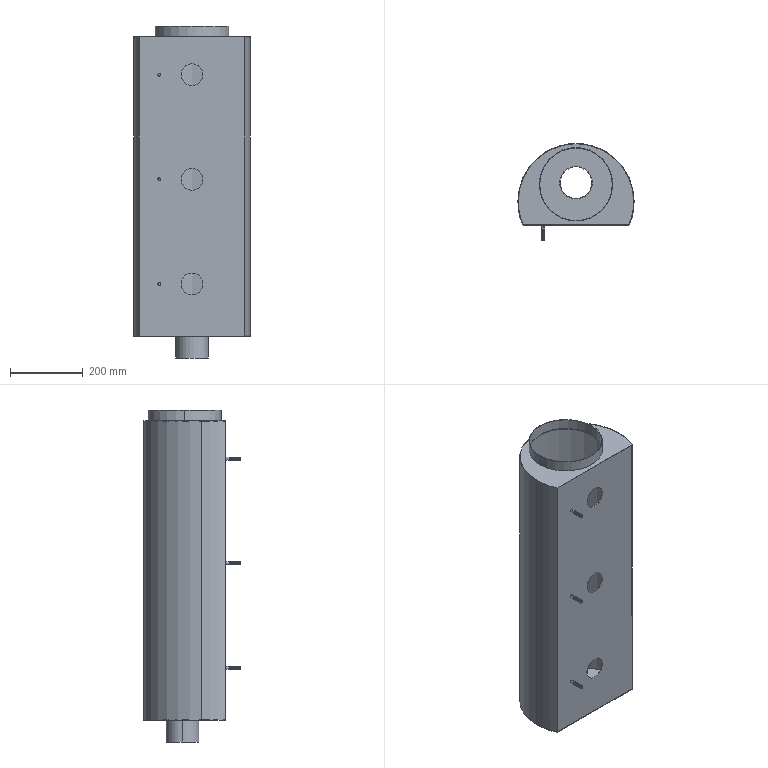Part | SolidWorks | features ICE 8, SweepThread 3, Extrusion 1, Shell 1 | 1 solid | 232 faces | box 320 x 266 x 914 mm | volume 1052652 mm3 | cylinder 206 | plane 17 | spline 9 | commonest cylinder face diameters 8 x186 60 x6 317.6 x3 320 x3 87.6 x2 90 x2